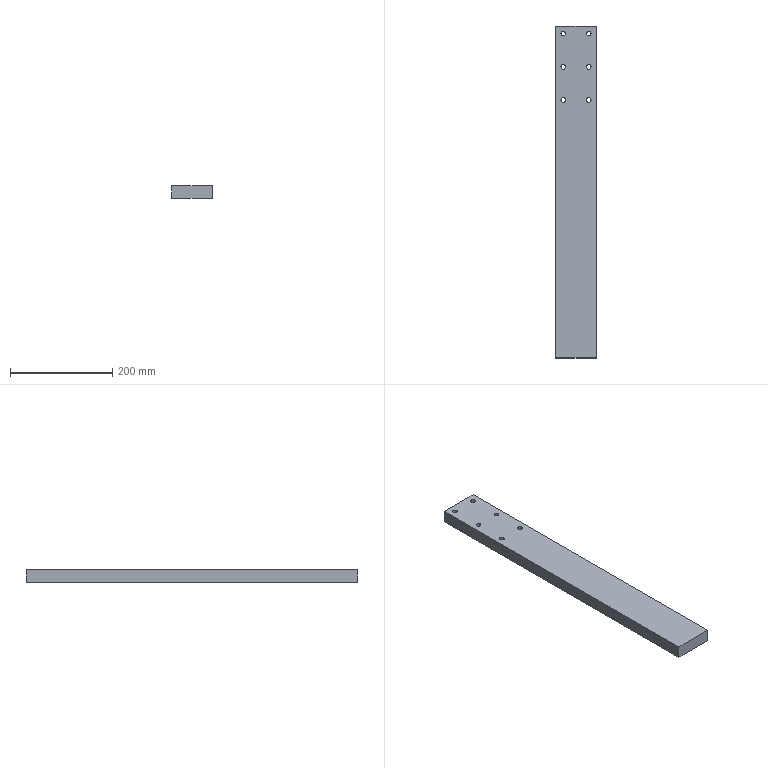Part | SolidWorks | features HoleWzd 2, 3DProfileFeature 1, Extrusion 1, LPattern 1 | 1 solid | 34 faces | box 80 x 650 x 25 mm | volume 1287489 mm3 | cylinder 20 | cone 8 | plane 6 | commonest cylinder face diameters 9 x12 6.8 x8
STEP:
#1=CARTESIAN_POINT('',(60.25,285.,15.9));
#2=VERTEX_POINT('',#1);
#3=CARTESIAN_POINT('',(60.25,285.,9.1));
#4=VERTEX_POINT('',#3);
#5=CARTESIAN_POINT('',(60.25,285.,12.5));
#6=DIRECTION('',(1.,0.,0.));
#7=DIRECTION('',(0.,0.,-1.));
#8=AXIS2_PLACEMENT_3D('',#5,#6,#7);
#9=CIRCLE('',#8,3.4);
#10=EDGE_CURVE('',#2,#4,#9,.T.);
#11=ORIENTED_EDGE('',*,*,#10,.F.);
#12=CARTESIAN_POINT('',(80.,285.,15.9));
#13=VERTEX_POINT('',#12);
#14=CARTESIAN_POINT('',(80.,285.,15.9));
#15=DIRECTION('',(1.,0.,0.));
#16=VECTOR('',#15,1000.);
#17=LINE('',#14,#16);
#18=EDGE_CURVE('',#2,#13,#17,.T.);
#19=ORIENTED_EDGE('',*,*,#18,.T.);
#20=CARTESIAN_POINT('',(80.,285.,9.1));
#21=VERTEX_POINT('',#20);
#22=CARTESIAN_POINT('',(80.,285.,12.5));
#23=DIRECTION('',(1.,0.,0.));
#24=DIRECTION('',(0.,0.,-1.));
#25=AXIS2_PLACEMENT_3D('',#22,#23,#24);
#26=CIRCLE('',#25,3.4);
#27=EDGE_CURVE('',#13,#21,#26,.T.);
#28=ORIENTED_EDGE('',*,*,#27,.T.);
#29=CARTESIAN_POINT('',(80.,285.,9.1));
#30=DIRECTION('',(1.,0.,0.));
#31=VECTOR('',#30,1000.);
#32=LINE('',#29,#31);
#33=EDGE_CURVE('',#4,#21,#32,.T.);
#34=ORIENTED_EDGE('',*,*,#33,.F.);
#35=EDGE_LOOP('',(#11,#19,#28,#34));
#36=FACE_OUTER_BOUND('',#35,.T.);
#37=CARTESIAN_POINT('',(80.,285.,12.5));
#38=DIRECTION('',(1.,0.,0.));
#39=DIRECTION('',(0.,0.,-1.));
#40=AXIS2_PLACEMENT_3D('',#37,#38,#39);
#41=CYLINDRICAL_SURFACE('',#40,3.4);
#42=ADVANCED_FACE('',(#36),#41,.F.);
#43=CARTESIAN_POINT('',(58.207,285.,12.5));
#44=VERTEX_POINT('',#43);
#45=CARTESIAN_POINT('',(60.25,285.,9.1));
#46=DIRECTION('',(0.515,0.,-0.8572));
#47=VECTOR('',#46,1000.);
#48=LINE('',#45,#47);
#49=EDGE_CURVE('',#44,#4,#48,.T.);
#50=ORIENTED_EDGE('',*,*,#49,.F.);
#51=CARTESIAN_POINT('',(60.25,285.,15.9));
#52=DIRECTION('',(0.515,0.,0.8572));
#53=VECTOR('',#52,1000.);
#54=LINE('',#51,#53);
#55=EDGE_CURVE('',#44,#2,#54,.T.);
#56=ORIENTED_EDGE('',*,*,#55,.T.);
#57=ORIENTED_EDGE('',*,*,#10,.T.);
#58=EDGE_LOOP('',(#50,#56,#57));
#59=FACE_OUTER_BOUND('',#58,.T.);
#60=CARTESIAN_POINT('',(60.25,285.,12.5));
#61=DIRECTION('',(1.,0.,0.));
#62=DIRECTION('',(0.,0.,-1.));
#63=AXIS2_PLACEMENT_3D('',#60,#61,#62);
#64=CONICAL_SURFACE('',#63,3.4,1.03);
#65=ADVANCED_FACE('',(#59),#64,.F.);
#66=CARTESIAN_POINT('',(60.25,320.,15.9));
#67=VERTEX_POINT('',#66);
#68=CARTESIAN_POINT('',(60.25,320.,9.1));
#69=VERTEX_POINT('',#68);
#70=CARTESIAN_POINT('',(60.25,320.,12.5));
#71=DIRECTION('',(1.,0.,0.));
#72=DIRECTION('',(0.,0.,-1.));
#73=AXIS2_PLACEMENT_3D('',#70,#71,#72);
#74=CIRCLE('',#73,3.4);
#75=EDGE_CURVE('',#67,#69,#74,.T.);
#76=ORIENTED_EDGE('',*,*,#75,.F.);
#77=CARTESIAN_POINT('',(80.,320.,15.9));
#78=VERTEX_POINT('',#77);
#79=CARTESIAN_POINT('',(80.,320.,15.9));
#80=DIRECTION('',(1.,0.,0.));
#81=VECTOR('',#80,1000.);
#82=LINE('',#79,#81);
#83=EDGE_CURVE('',#67,#78,#82,.T.);
#84=ORIENTED_EDGE('',*,*,#83,.T.);
#85=CARTESIAN_POINT('',(80.,320.,9.1));
#86=VERTEX_POINT('',#85);
#87=CARTESIAN_POINT('',(80.,320.,12.5));
#88=DIRECTION('',(1.,0.,0.));
#89=DIRECTION('',(0.,0.,-1.));
#90=AXIS2_PLACEMENT_3D('',#87,#88,#89);
#91=CIRCLE('',#90,3.4);
#92=EDGE_CURVE('',#78,#86,#91,.T.);
#93=ORIENTED_EDGE('',*,*,#92,.T.);
#94=CARTESIAN_POINT('',(80.,320.,9.1));
#95=DIRECTION('',(1.,0.,0.));
#96=VECTOR('',#95,1000.);
#97=LINE('',#94,#96);
#98=EDGE_CURVE('',#69,#86,#97,.T.);
#99=ORIENTED_EDGE('',*,*,#98,.F.);
#100=EDGE_LOOP('',(#76,#84,#93,#99));
#101=FACE_OUTER_BOUND('',#100,.T.);
#102=CARTESIAN_POINT('',(80.,320.,12.5));
#103=DIRECTION('',(1.,0.,0.));
#104=DIRECTION('',(0.,0.,-1.));
#105=AXIS2_PLACEMENT_3D('',#102,#103,#104);
#106=CYLINDRICAL_SURFACE('',#105,3.4);
#107=ADVANCED_FACE('',(#101),#106,.F.);
#108=CARTESIAN_POINT('',(58.207,320.,12.5));
#109=VERTEX_POINT('',#108);
#110=CARTESIAN_POINT('',(60.25,320.,9.1));
#111=DIRECTION('',(0.515,0.,-0.8572));
#112=VECTOR('',#111,1000.);
#113=LINE('',#110,#112);
#114=EDGE_CURVE('',#109,#69,#113,.T.);
#115=ORIENTED_EDGE('',*,*,#114,.F.);
#116=CARTESIAN_POINT('',(60.25,320.,15.9));
#117=DIRECTION('',(0.515,0.,0.8572));
#118=VECTOR('',#117,1000.);
#119=LINE('',#116,#118);
#120=EDGE_CURVE('',#109,#67,#119,.T.);
#121=ORIENTED_EDGE('',*,*,#120,.T.);
#122=ORIENTED_EDGE('',*,*,#75,.T.);
#123=EDGE_LOOP('',(#115,#121,#122));
#124=FACE_OUTER_BOUND('',#123,.T.);
#125=CARTESIAN_POINT('',(60.25,320.,12.5));
#126=DIRECTION('',(1.,0.,0.));
#127=DIRECTION('',(0.,0.,-1.));
#128=AXIS2_PLACEMENT_3D('',#125,#126,#127);
#129=CONICAL_SURFACE('',#128,3.4,1.03);
#130=ADVANCED_FACE('',(#124),#129,.F.);
#131=CARTESIAN_POINT('',(60.25,620.,15.9));
#132=VERTEX_POINT('',#131);
#133=CARTESIAN_POINT('',(60.25,620.,9.1));
#134=VERTEX_POINT('',#133);
#135=CARTESIAN_POINT('',(60.25,620.,12.5));
#136=DIRECTION('',(1.,0.,0.));
#137=DIRECTION('',(0.,0.,-1.));
#138=AXIS2_PLACEMENT_3D('',#135,#136,#137);
#139=CIRCLE('',#138,3.4);
#140=EDGE_CURVE('',#132,#134,#139,.T.);
#141=ORIENTED_EDGE('',*,*,#140,.F.);
#142=CARTESIAN_POINT('',(80.,620.,15.9));
#143=VERTEX_POINT('',#142);
#144=CARTESIAN_POINT('',(80.,620.,15.9));
#145=DIRECTION('',(1.,0.,0.));
#146=VECTOR('',#145,1000.);
#147=LINE('',#144,#146);
#148=EDGE_CURVE('',#132,#143,#147,.T.);
#149=ORIENTED_EDGE('',*,*,#148,.T.);
#150=CARTESIAN_POINT('',(80.,620.,9.1));
#151=VERTEX_POINT('',#150);
#152=CARTESIAN_POINT('',(80.,620.,12.5));
#153=DIRECTION('',(1.,0.,0.));
#154=DIRECTION('',(0.,0.,-1.));
#155=AXIS2_PLACEMENT_3D('',#152,#153,#154);
#156=CIRCLE('',#155,3.4);
#157=EDGE_CURVE('',#143,#151,#156,.T.);
#158=ORIENTED_EDGE('',*,*,#157,.T.);
#159=CARTESIAN_POINT('',(80.,620.,9.1));
#160=DIRECTION('',(1.,0.,0.));
#161=VECTOR('',#160,1000.);
#162=LINE('',#159,#161);
#163=EDGE_CURVE('',#134,#151,#162,.T.);
#164=ORIENTED_EDGE('',*,*,#163,.F.);
#165=EDGE_LOOP('',(#141,#149,#158,#164));
#166=FACE_OUTER_BOUND('',#165,.T.);
#167=CARTESIAN_POINT('',(80.,620.,12.5));
#168=DIRECTION('',(1.,0.,0.));
#169=DIRECTION('',(0.,0.,-1.));
#170=AXIS2_PLACEMENT_3D('',#167,#168,#169);
#171=CYLINDRICAL_SURFACE('',#170,3.4);
#172=ADVANCED_FACE('',(#166),#171,.F.);
#173=CARTESIAN_POINT('',(58.207,620.,12.5));
#174=VERTEX_POINT('',#173);
#175=CARTESIAN_POINT('',(60.25,620.,9.1));
#176=DIRECTION('',(0.515,0.,-0.8572));
#177=VECTOR('',#176,1000.);
#178=LINE('',#175,#177);
#179=EDGE_CURVE('',#174,#134,#178,.T.);
#180=ORIENTED_EDGE('',*,*,#179,.F.);
#181=CARTESIAN_POINT('',(60.25,620.,15.9));
#182=DIRECTION('',(0.515,0.,0.8572));
#183=VECTOR('',#182,1000.);
#184=LINE('',#181,#183);
#185=EDGE_CURVE('',#174,#132,#184,.T.);
#186=ORIENTED_EDGE('',*,*,#185,.T.);
#187=ORIENTED_EDGE('',*,*,#140,.T.);
#188=EDGE_LOOP('',(#180,#186,#187));
#189=FACE_OUTER_BOUND('',#188,.T.);
#190=CARTESIAN_POINT('',(60.25,620.,12.5));
#191=DIRECTION('',(1.,0.,0.));
#192=DIRECTION('',(0.,0.,-1.));
#193=AXIS2_PLACEMENT_3D('',#190,#191,#192);
#194=CONICAL_SURFACE('',#193,3.4,1.03);
#195=ADVANCED_FACE('',(#189),#194,.F.);
#196=CARTESIAN_POINT('',(60.25,585.,15.9));
#197=VERTEX_POINT('',#196);
#198=CARTESIAN_POINT('',(60.25,585.,9.1));
#199=VERTEX_POINT('',#198);
#200=CARTESIAN_POINT('',(60.25,585.,12.5));
#201=DIRECTION('',(1.,0.,0.));
#202=DIRECTION('',(0.,0.,-1.));
#203=AXIS2_PLACEMENT_3D('',#200,#201,#202);
#204=CIRCLE('',#203,3.4);
#205=EDGE_CURVE('',#197,#199,#204,.T.);
#206=ORIENTED_EDGE('',*,*,#205,.F.);
#207=CARTESIAN_POINT('',(80.,585.,15.9));
#208=VERTEX_POINT('',#207);
#209=CARTESIAN_POINT('',(80.,585.,15.9));
#210=DIRECTION('',(1.,0.,0.));
#211=VECTOR('',#210,1000.);
#212=LINE('',#209,#211);
#213=EDGE_CURVE('',#197,#208,#212,.T.);
#214=ORIENTED_EDGE('',*,*,#213,.T.);
#215=CARTESIAN_POINT('',(80.,585.,9.1));
#216=VERTEX_POINT('',#215);
#217=CARTESIAN_POINT('',(80.,585.,12.5));
#218=DIRECTION('',(1.,0.,0.));
#219=DIRECTION('',(0.,0.,-1.));
#220=AXIS2_PLACEMENT_3D('',#217,#218,#219);
#221=CIRCLE('',#220,3.4);
#222=EDGE_CURVE('',#208,#216,#221,.T.);
#223=ORIENTED_EDGE('',*,*,#222,.T.);
#224=CARTESIAN_POINT('',(80.,585.,9.1));
#225=DIRECTION('',(1.,0.,0.));
#226=VECTOR('',#225,1000.);
#227=LINE('',#224,#226);
#228=EDGE_CURVE('',#199,#216,#227,.T.);
#229=ORIENTED_EDGE('',*,*,#228,.F.);
#230=EDGE_LOOP('',(#206,#214,#223,#229));
#231=FACE_OUTER_BOUND('',#230,.T.);
#232=CARTESIAN_POINT('',(80.,585.,12.5));
#233=DIRECTION('',(1.,0.,0.));
#234=DIRECTION('',(0.,0.,-1.));
#235=AXIS2_PLACEMENT_3D('',#232,#233,#234);
#236=CYLINDRICAL_SURFACE('',#235,3.4);
#237=ADVANCED_FACE('',(#231),#236,.F.);
#238=CARTESIAN_POINT('',(58.207,585.,12.5));
#239=VERTEX_POINT('',#238);
#240=CARTESIAN_POINT('',(60.25,585.,9.1));
#241=DIRECTION('',(0.515,0.,-0.8572));
#242=VECTOR('',#241,1000.);
#243=LINE('',#240,#242);
#244=EDGE_CURVE('',#239,#199,#243,.T.);
#245=ORIENTED_EDGE('',*,*,#244,.F.);
#246=CARTESIAN_POINT('',(60.25,585.,15.9));
#247=DIRECTION('',(0.515,0.,0.8572));
#248=VECTOR('',#247,1000.);
#249=LINE('',#246,#248);
#250=EDGE_CURVE('',#239,#197,#249,.T.);
#251=ORIENTED_EDGE('',*,*,#250,.T.);
#252=ORIENTED_EDGE('',*,*,#205,.T.);
#253=EDGE_LOOP('',(#245,#251,#252));
#254=FACE_OUTER_BOUND('',#253,.T.);
#255=CARTESIAN_POINT('',(60.25,585.,12.5));
#256=DIRECTION('',(1.,0.,0.));
#257=DIRECTION('',(0.,0.,-1.));
#258=AXIS2_PLACEMENT_3D('',#255,#256,#257);
#259=CONICAL_SURFACE('',#258,3.4,1.03);
#260=ADVANCED_FACE('',(#254),#259,.F.);
#261=CARTESIAN_POINT('',(10.5,635.,0.));
#262=VERTEX_POINT('',#261);
#263=CARTESIAN_POINT('',(19.5,635.,0.));
#264=VERTEX_POINT('',#263);
#265=CARTESIAN_POINT('',(15.,635.,0.));
#266=DIRECTION('',(0.,0.,1.));
#267=DIRECTION('',(1.,0.,0.));
#268=AXIS2_PLACEMENT_3D('',#265,#266,#267);
#269=CIRCLE('',#268,4.5);
#270=EDGE_CURVE('',#262,#264,#269,.T.);
#271=ORIENTED_EDGE('',*,*,#270,.F.);
#272=CARTESIAN_POINT('',(10.5,635.,25.));
#273=VERTEX_POINT('',#272);
#274=CARTESIAN_POINT('',(10.5,635.,25.));
#275=DIRECTION('',(0.,0.,1.));
#276=VECTOR('',#275,1000.);
#277=LINE('',#274,#276);
#278=EDGE_CURVE('',#262,#273,#277,.T.);
#279=ORIENTED_EDGE('',*,*,#278,.T.);
#280=CARTESIAN_POINT('',(19.5,635.,25.));
#281=VERTEX_POINT('',#280);
#282=CARTESIAN_POINT('',(15.,635.,25.));
#283=DIRECTION('',(0.,0.,1.));
#284=DIRECTION('',(1.,0.,0.));
#285=AXIS2_PLACEMENT_3D('',#282,#283,#284);
#286=CIRCLE('',#285,4.5);
#287=EDGE_CURVE('',#273,#281,#286,.T.);
#288=ORIENTED_EDGE('',*,*,#287,.T.);
#289=CARTESIAN_POINT('',(19.5,635.,25.));
#290=DIRECTION('',(0.,0.,1.));
#291=VECTOR('',#290,1000.);
#292=LINE('',#289,#291);
#293=EDGE_CURVE('',#264,#281,#292,.T.);
#294=ORIENTED_EDGE('',*,*,#293,.F.);
#295=EDGE_LOOP('',(#271,#279,#288,#294));
#296=FACE_OUTER_BOUND('',#295,.T.);
#297=CARTESIAN_POINT('',(15.,635.,25.));
#298=DIRECTION('',(0.,0.,1.));
#299=DIRECTION('',(1.,0.,0.));
#300=AXIS2_PLACEMENT_3D('',#297,#298,#299);
#301=CYLINDRICAL_SURFACE('',#300,4.5);
#302=ADVANCED_FACE('',(#296),#301,.F.);
#303=CARTESIAN_POINT('',(60.5,635.,0.));
#304=VERTEX_POINT('',#303);
#305=CARTESIAN_POINT('',(69.5,635.,0.));
#306=VERTEX_POINT('',#305);
#307=CARTESIAN_POINT('',(65.,635.,0.));
#308=DIRECTION('',(0.,0.,1.));
#309=DIRECTION('',(1.,0.,0.));
#310=AXIS2_PLACEMENT_3D('',#307,#308,#309);
#311=CIRCLE('',#310,4.5);
#312=EDGE_CURVE('',#304,#306,#311,.T.);
#313=ORIENTED_EDGE('',*,*,#312,.F.);
#314=CARTESIAN_POINT('',(60.5,635.,25.));
#315=VERTEX_POINT('',#314);
#316=CARTESIAN_POINT('',(60.5,635.,25.));
#317=DIRECTION('',(0.,0.,1.));
#318=VECTOR('',#317,1000.);
#319=LINE('',#316,#318);
#320=EDGE_CURVE('',#304,#315,#319,.T.);
#321=ORIENTED_EDGE('',*,*,#320,.T.);
#322=CARTESIAN_POINT('',(69.5,635.,25.));
#323=VERTEX_POINT('',#322);
#324=CARTESIAN_POINT('',(65.,635.,25.));
#325=DIRECTION('',(0.,0.,1.));
#326=DIRECTION('',(1.,0.,0.));
#327=AXIS2_PLACEMENT_3D('',#324,#325,#326);
#328=CIRCLE('',#327,4.5);
#329=EDGE_CURVE('',#315,#323,#328,.T.);
#330=ORIENTED_EDGE('',*,*,#329,.T.);
#331=CARTESIAN_POINT('',(69.5,635.,25.));
#332=DIRECTION('',(0.,0.,1.));
#333=VECTOR('',#332,1000.);
#334=LINE('',#331,#333);
#335=EDGE_CURVE('',#306,#323,#334,.T.);
#336=ORIENTED_EDGE('',*,*,#335,.F.);
#337=EDGE_LOOP('',(#313,#321,#330,#336));
#338=FACE_OUTER_BOUND('',#337,.T.);
#339=CARTESIAN_POINT('',(65.,635.,25.));
#340=DIRECTION('',(0.,0.,1.));
#341=DIRECTION('',(1.,0.,0.));
#342=AXIS2_PLACEMENT_3D('',#339,#340,#341);
#343=CYLINDRICAL_SURFACE('',#342,4.5);
#344=ADVANCED_FACE('',(#338),#343,.F.);
#345=CARTESIAN_POINT('',(10.5,505.,0.));
#346=VERTEX_POINT('',#345);
#347=CARTESIAN_POINT('',(19.5,505.,0.));
#348=VERTEX_POINT('',#347);
#349=CARTESIAN_POINT('',(15.,505.,0.));
#350=DIRECTION('',(0.,0.,1.));
#351=DIRECTION('',(1.,0.,0.));
#352=AXIS2_PLACEMENT_3D('',#349,#350,#351);
#353=CIRCLE('',#352,4.5);
#354=EDGE_CURVE('',#346,#348,#353,.T.);
#355=ORIENTED_EDGE('',*,*,#354,.F.);
#356=CARTESIAN_POINT('',(10.5,505.,25.));
#357=VERTEX_POINT('',#356);
#358=CARTESIAN_POINT('',(10.5,505.,25.));
#359=DIRECTION('',(0.,0.,1.));
#360=VECTOR('',#359,1000.);
#361=LINE('',#358,#360);
#362=EDGE_CURVE('',#346,#357,#361,.T.);
#363=ORIENTED_EDGE('',*,*,#362,.T.);
#364=CARTESIAN_POINT('',(19.5,505.,25.));
#365=VERTEX_POINT('',#364);
#366=CARTESIAN_POINT('',(15.,505.,25.));
#367=DIRECTION('',(0.,0.,1.));
#368=DIRECTION('',(1.,0.,0.));
#369=AXIS2_PLACEMENT_3D('',#366,#367,#368);
#370=CIRCLE('',#369,4.5);
#371=EDGE_CURVE('',#357,#365,#370,.T.);
#372=ORIENTED_EDGE('',*,*,#371,.T.);
#373=CARTESIAN_POINT('',(19.5,505.,25.));
#374=DIRECTION('',(0.,0.,1.));
#375=VECTOR('',#374,1000.);
#376=LINE('',#373,#375);
#377=EDGE_CURVE('',#348,#365,#376,.T.);
#378=ORIENTED_EDGE('',*,*,#377,.F.);
#379=EDGE_LOOP('',(#355,#363,#372,#378));
#380=FACE_OUTER_BOUND('',#379,.T.);
#381=CARTESIAN_POINT('',(15.,505.,25.));
#382=DIRECTION('',(0.,0.,1.));
#383=DIRECTION('',(1.,0.,0.));
#384=AXIS2_PLACEMENT_3D('',#381,#382,#383);
#385=CYLINDRICAL_SURFACE('',#384,4.5);
#386=ADVANCED_FACE('',(#380),#385,.F.);
#387=CARTESIAN_POINT('',(60.5,505.,0.));
#388=VERTEX_POINT('',#387);
#389=CARTESIAN_POINT('',(69.5,505.,0.));
#390=VERTEX_POINT('',#389);
#391=CARTESIAN_POINT('',(65.,505.,0.));
#392=DIRECTION('',(0.,0.,1.));
#393=DIRECTION('',(1.,0.,0.));
#394=AXIS2_PLACEMENT_3D('',#391,#392,#393);
#395=CIRCLE('',#394,4.5);
#396=EDGE_CURVE('',#388,#390,#395,.T.);
#397=ORIENTED_EDGE('',*,*,#396,.F.);
#398=CARTESIAN_POINT('',(60.5,505.,25.));
#399=VERTEX_POINT('',#398);
#400=CARTESIAN_POINT('',(60.5,505.,25.));
#401=DIRECTION('',(0.,0.,1.));
#402=VECTOR('',#401,1000.);
#403=LINE('',#400,#402);
#404=EDGE_CURVE('',#388,#399,#403,.T.);
#405=ORIENTED_EDGE('',*,*,#404,.T.);
#406=CARTESIAN_POINT('',(69.5,505.,25.));
#407=VERTEX_POINT('',#406);
#408=CARTESIAN_POINT('',(65.,505.,25.));
#409=DIRECTION('',(0.,0.,1.));
#410=DIRECTION('',(1.,0.,0.));
#411=AXIS2_PLACEMENT_3D('',#408,#409,#410);
#412=CIRCLE('',#411,4.5);
#413=EDGE_CURVE('',#399,#407,#412,.T.);
#414=ORIENTED_EDGE('',*,*,#413,.T.);
#415=CARTESIAN_POINT('',(69.5,505.,25.));
#416=DIRECTION('',(0.,0.,1.));
#417=VECTOR('',#416,1000.);
#418=LINE('',#415,#417);
#419=EDGE_CURVE('',#390,#407,#418,.T.);
#420=ORIENTED_EDGE('',*,*,#419,.F.);
#421=EDGE_LOOP('',(#397,#405,#414,#420));
#422=FACE_OUTER_BOUND('',#421,.T.);
#423=CARTESIAN_POINT('',(65.,505.,25.));
#424=DIRECTION('',(0.,0.,1.));
#425=DIRECTION('',(1.,0.,0.));
#426=AXIS2_PLACEMENT_3D('',#423,#424,#425);
#427=CYLINDRICAL_SURFACE('',#426,4.5);
#428=ADVANCED_FACE('',(#422),#427,.F.);
#429=CARTESIAN_POINT('',(10.5,570.,0.));
#430=VERTEX_POINT('',#429);
#431=CARTESIAN_POINT('',(19.5,570.,0.));
#432=VERTEX_POINT('',#431);
#433=CARTESIAN_POINT('',(15.,570.,0.));
#434=DIRECTION('',(0.,0.,1.));
#435=DIRECTION('',(1.,0.,0.));
#436=AXIS2_PLACEMENT_3D('',#433,#434,#435);
#437=CIRCLE('',#436,4.5);
#438=EDGE_CURVE('',#430,#432,#437,.T.);
#439=ORIENTED_EDGE('',*,*,#438,.F.);
#440=CARTESIAN_POINT('',(10.5,570.,25.));
#441=VERTEX_POINT('',#440);
#442=CARTESIAN_POINT('',(10.5,570.,25.));
#443=DIRECTION('',(0.,0.,1.));
#444=VECTOR('',#443,1000.);
#445=LINE('',#442,#444);
#446=EDGE_CURVE('',#430,#441,#445,.T.);
#447=ORIENTED_EDGE('',*,*,#446,.T.);
#448=CARTESIAN_POINT('',(19.5,570.,25.));
#449=VERTEX_POINT('',#448);
#450=CARTESIAN_POINT('',(15.,570.,25.));
#451=DIRECTION('',(0.,0.,1.));
#452=DIRECTION('',(1.,0.,0.));
#453=AXIS2_PLACEMENT_3D('',#450,#451,#452);
#454=CIRCLE('',#453,4.5);
#455=EDGE_CURVE('',#441,#449,#454,.T.);
#456=ORIENTED_EDGE('',*,*,#455,.T.);
#457=CARTESIAN_POINT('',(19.5,570.,25.));
#458=DIRECTION('',(0.,0.,1.));
#459=VECTOR('',#458,1000.);
#460=LINE('',#457,#459);
#461=EDGE_CURVE('',#432,#449,#460,.T.);
#462=ORIENTED_EDGE('',*,*,#461,.F.);
#463=EDGE_LOOP('',(#439,#447,#456,#462));
#464=FACE_OUTER_BOUND('',#463,.T.);
#465=CARTESIAN_POINT('',(15.,570.,25.));
#466=DIRECTION('',(0.,0.,1.));
#467=DIRECTION('',(1.,0.,0.));
#468=AXIS2_PLACEMENT_3D('',#465,#466,#467);
#469=CYLINDRICAL_SURFACE('',#468,4.5);
#470=ADVANCED_FACE('',(#464),#469,.F.);
#471=CARTESIAN_POINT('',(60.5,570.,0.));
#472=VERTEX_POINT('',#471);
#473=CARTESIAN_POINT('',(69.5,570.,0.));
#474=VERTEX_POINT('',#473);
#475=CARTESIAN_POINT('',(65.,570.,0.));
#476=DIRECTION('',(0.,0.,1.));
#477=DIRECTION('',(1.,0.,0.));
#478=AXIS2_PLACEMENT_3D('',#475,#476,#477);
#479=CIRCLE('',#478,4.5);
#480=EDGE_CURVE('',#472,#474,#479,.T.);
#481=ORIENTED_EDGE('',*,*,#480,.F.);
#482=CARTESIAN_POINT('',(60.5,570.,25.));
#483=VERTEX_POINT('',#482);
#484=CARTESIAN_POINT('',(60.5,570.,25.));
#485=DIRECTION('',(0.,0.,1.));
#486=VECTOR('',#485,1000.);
#487=LINE('',#484,#486);
#488=EDGE_CURVE('',#472,#483,#487,.T.);
#489=ORIENTED_EDGE('',*,*,#488,.T.);
#490=CARTESIAN_POINT('',(69.5,570.,25.));
#491=VERTEX_POINT('',#490);
#492=CARTESIAN_POINT('',(65.,570.,25.));
#493=DIRECTION('',(0.,0.,1.));
#494=DIRECTION('',(1.,0.,0.));
#495=AXIS2_PLACEMENT_3D('',#492,#493,#494);
#496=CIRCLE('',#495,4.5);
#497=EDGE_CURVE('',#483,#491,#496,.T.);
#498=ORIENTED_EDGE('',*,*,#497,.T.);
#499=CARTESIAN_POINT('',(69.5,570.,25.));
#500=DIRECTION('',(0.,0.,1.));
#501=VECTOR('',#500,1000.);
#502=LINE('',#499,#501);
#503=EDGE_CURVE('',#474,#491,#502,.T.);
#504=ORIENTED_EDGE('',*,*,#503,.F.);
#505=EDGE_LOOP('',(#481,#489,#498,#504));
#506=FACE_OUTER_BOUND('',#505,.T.);
#507=CARTESIAN_POINT('',(65.,570.,25.));
#508=DIRECTION('',(0.,0.,1.));
#509=DIRECTION('',(1.,0.,0.));
#510=AXIS2_PLACEMENT_3D('',#507,#508,#509);
#511=CYLINDRICAL_SURFACE('',#510,4.5);
#512=ADVANCED_FACE('',(#506),#511,.F.);
#513=CARTESIAN_POINT('',(0.,650.,0.));
#514=VERTEX_POINT('',#513);
#515=CARTESIAN_POINT('',(0.,0.,0.));
#516=VERTEX_POINT('',#515);
#517=CARTESIAN_POINT('',(0.,0.,0.));
#518=DIRECTION('',(0.,-1.,0.));
#519=VECTOR('',#518,1000.);
#520=LINE('',#517,#519);
#521=EDGE_CURVE('',#514,#516,#520,.T.);
#522=ORIENTED_EDGE('',*,*,#521,.T.);
#523=CARTESIAN_POINT('',(0.,0.,25.));
#524=VERTEX_POINT('',#523);
#525=CARTESIAN_POINT('',(0.,0.,25.));
#526=DIRECTION('',(0.,0.,-1.));
#527=VECTOR('',#526,1000.);
#528=LINE('',#525,#527);
#529=EDGE_CURVE('',#524,#516,#528,.T.);
#530=ORIENTED_EDGE('',*,*,#529,.F.);
#531=CARTESIAN_POINT('',(0.,650.,25.));
#532=VERTEX_POINT('',#531);
#533=CARTESIAN_POINT('',(0.,0.,25.));
#534=DIRECTION('',(0.,-1.,0.));
#535=VECTOR('',#534,1000.);
#536=LINE('',#533,#535);
#537=EDGE_CURVE('',#532,#524,#536,.T.);
#538=ORIENTED_EDGE('',*,*,#537,.F.);
#539=CARTESIAN_POINT('',(0.,650.,25.));
#540=DIRECTION('',(0.,0.,-1.));
#541=VECTOR('',#540,1000.);
#542=LINE('',#539,#541);
#543=EDGE_CURVE('',#532,#514,#542,.T.);
#544=ORIENTED_EDGE('',*,*,#543,.T.);
#545=EDGE_LOOP('',(#522,#530,#538,#544));
#546=FACE_OUTER_BOUND('',#545,.T.);
#547=CARTESIAN_POINT('',(0.,0.,25.));
#548=DIRECTION('',(1.,0.,0.));
#549=DIRECTION('',(0.,0.,-1.));
#550=AXIS2_PLACEMENT_3D('',#547,#548,#549);
#551=PLANE('',#550);
#552=ADVANCED_FACE('',(#546),#551,.F.);
#553=CARTESIAN_POINT('',(80.,0.,0.));
#554=VERTEX_POINT('',#553);
#555=CARTESIAN_POINT('',(0.,0.,0.));
#556=DIRECTION('',(1.,0.,0.));
#557=VECTOR('',#556,1000.);
#558=LINE('',#555,#557);
#559=EDGE_CURVE('',#516,#554,#558,.T.);
#560=ORIENTED_EDGE('',*,*,#559,.T.);
#561=CARTESIAN_POINT('',(80.,0.,25.));
#562=VERTEX_POINT('',#561);
#563=CARTESIAN_POINT('',(80.,0.,25.));
#564=DIRECTION('',(0.,0.,-1.));
#565=VECTOR('',#564,1000.);
#566=LINE('',#563,#565);
#567=EDGE_CURVE('',#562,#554,#566,.T.);
#568=ORIENTED_EDGE('',*,*,#567,.F.);
#569=CARTESIAN_POINT('',(0.,0.,25.));
#570=DIRECTION('',(1.,0.,0.));
#571=VECTOR('',#570,1000.);
#572=LINE('',#569,#571);
#573=EDGE_CURVE('',#524,#562,#572,.T.);
#574=ORIENTED_EDGE('',*,*,#573,.F.);
#575=ORIENTED_EDGE('',*,*,#529,.T.);
#576=EDGE_LOOP('',(#560,#568,#574,#575));
#577=FACE_OUTER_BOUND('',#576,.T.);
#578=CARTESIAN_POINT('',(0.,0.,25.));
#579=DIRECTION('',(0.,1.,0.));
#580=DIRECTION('',(0.,0.,1.));
#581=AXIS2_PLACEMENT_3D('',#578,#579,#580);
#582=PLANE('',#581);
#583=ADVANCED_FACE('',(#577),#582,.F.);
#584=CARTESIAN_POINT('',(80.,285.,12.5));
#585=DIRECTION('',(1.,0.,0.));
#586=DIRECTION('',(0.,0.,-1.));
#587=AXIS2_PLACEMENT_3D('',#584,#585,#586);
#588=CIRCLE('',#587,3.4);
#589=EDGE_CURVE('',#21,#13,#588,.T.);
#590=ORIENTED_EDGE('',*,*,#589,.F.);
#591=ORIENTED_EDGE('',*,*,#27,.F.);
#592=EDGE_LOOP('',(#590,#591));
#593=FACE_BOUND('',#592,.T.);
#594=CARTESIAN_POINT('',(80.,320.,12.5));
#595=DIRECTION('',(1.,0.,0.));
#596=DIRECTION('',(0.,0.,-1.));
#597=AXIS2_PLACEMENT_3D('',#594,#595,#596);
#598=CIRCLE('',#597,3.4);
#599=EDGE_CURVE('',#86,#78,#598,.T.);
#600=ORIENTED_EDGE('',*,*,#599,.F.);
#601=ORIENTED_EDGE('',*,*,#92,.F.);
#602=EDGE_LOOP('',(#600,#601));
#603=FACE_BOUND('',#602,.T.);
#604=CARTESIAN_POINT('',(80.,620.,12.5));
#605=DIRECTION('',(1.,0.,0.));
#606=DIRECTION('',(0.,0.,-1.));
#607=AXIS2_PLACEMENT_3D('',#604,#605,#606);
#608=CIRCLE('',#607,3.4);
#609=EDGE_CURVE('',#151,#143,#608,.T.);
#610=ORIENTED_EDGE('',*,*,#609,.F.);
#611=ORIENTED_EDGE('',*,*,#157,.F.);
#612=EDGE_LOOP('',(#610,#611));
#613=FACE_BOUND('',#612,.T.);
#614=CARTESIAN_POINT('',(80.,585.,12.5));
#615=DIRECTION('',(1.,0.,0.));
#616=DIRECTION('',(0.,0.,-1.));
#617=AXIS2_PLACEMENT_3D('',#614,#615,#616);
#618=CIRCLE('',#617,3.4);
#619=EDGE_CURVE('',#216,#208,#618,.T.);
#620=ORIENTED_EDGE('',*,*,#619,.F.);
#621=ORIENTED_EDGE('',*,*,#222,.F.);
#622=EDGE_LOOP('',(#620,#621));
#623=FACE_BOUND('',#622,.T.);
#624=CARTESIAN_POINT('',(80.,650.,0.));
#625=VERTEX_POINT('',#624);
#626=CARTESIAN_POINT('',(80.,80.,0.));
#627=DIRECTION('',(0.,1.,0.));
#628=VECTOR('',#627,1000.);
#629=LINE('',#626,#628);
#630=EDGE_CURVE('',#554,#625,#629,.T.);
#631=ORIENTED_EDGE('',*,*,#630,.T.);
#632=CARTESIAN_POINT('',(80.,650.,25.));
#633=VERTEX_POINT('',#632);
#634=CARTESIAN_POINT('',(80.,650.,25.));
#635=DIRECTION('',(0.,0.,-1.));
#636=VECTOR('',#635,1000.);
#637=LINE('',#634,#636);
#638=EDGE_CURVE('',#633,#625,#637,.T.);
#639=ORIENTED_EDGE('',*,*,#638,.F.);
#640=CARTESIAN_POINT('',(80.,0.,25.));
#641=DIRECTION('',(0.,1.,0.));
#642=VECTOR('',#641,1000.);
#643=LINE('',#640,#642);
#644=EDGE_CURVE('',#562,#633,#643,.T.);
#645=ORIENTED_EDGE('',*,*,#644,.F.);
#646=ORIENTED_EDGE('',*,*,#567,.T.);
#647=EDGE_LOOP('',(#631,#639,#645,#646));
#648=FACE_OUTER_BOUND('',#647,.T.);
#649=CARTESIAN_POINT('',(80.,80.,25.));
#650=DIRECTION('',(-1.,0.,0.));
#651=DIRECTION('',(0.,0.,1.));
#652=AXIS2_PLACEMENT_3D('',#649,#650,#651);
#653=PLANE('',#652);
#654=ADVANCED_FACE('',(#593,#603,#613,#623,#648),#653,.F.);
#655=CARTESIAN_POINT('',(0.,650.,0.));
#656=DIRECTION('',(-1.,0.,0.));
#657=VECTOR('',#656,1000.);
#658=LINE('',#655,#657);
#659=EDGE_CURVE('',#625,#514,#658,.T.);
#660=ORIENTED_EDGE('',*,*,#659,.T.);
#661=ORIENTED_EDGE('',*,*,#543,.F.);
#662=CARTESIAN_POINT('',(0.,650.,25.));
#663=DIRECTION('',(-1.,0.,0.));
#664=VECTOR('',#663,1000.);
#665=LINE('',#662,#664);
#666=EDGE_CURVE('',#633,#532,#665,.T.);
#667=ORIENTED_EDGE('',*,*,#666,.F.);
#668=ORIENTED_EDGE('',*,*,#638,.T.);
#669=EDGE_LOOP('',(#660,#661,#667,#668));
#670=FACE_OUTER_BOUND('',#669,.T.);
#671=CARTESIAN_POINT('',(0.,650.,25.));
#672=DIRECTION('',(0.,-1.,0.));
#673=DIRECTION('',(0.,0.,-1.));
#674=AXIS2_PLACEMENT_3D('',#671,#672,#673);
#675=PLANE('',#674);
#676=ADVANCED_FACE('',(#670),#675,.F.);
#677=CARTESIAN_POINT('',(15.,635.,25.));
#678=DIRECTION('',(0.,0.,1.));
#679=DIRECTION('',(1.,0.,0.));
#680=AXIS2_PLACEMENT_3D('',#677,#678,#679);
#681=CIRCLE('',#680,4.5);
#682=EDGE_CURVE('',#281,#273,#681,.T.);
#683=ORIENTED_EDGE('',*,*,#682,.F.);
#684=ORIENTED_EDGE('',*,*,#287,.F.);
#685=EDGE_LOOP('',(#683,#684));
#686=FACE_BOUND('',#685,.T.);
#687=CARTESIAN_POINT('',(65.,635.,25.));
#688=DIRECTION('',(0.,0.,1.));
#689=DIRECTION('',(1.,0.,0.));
#690=AXIS2_PLACEMENT_3D('',#687,#688,#689);
#691=CIRCLE('',#690,4.5);
#692=EDGE_CURVE('',#323,#315,#691,.T.);
#693=ORIENTED_EDGE('',*,*,#692,.F.);
#694=ORIENTED_EDGE('',*,*,#329,.F.);
#695=EDGE_LOOP('',(#693,#694));
#696=FACE_BOUND('',#695,.T.);
#697=CARTESIAN_POINT('',(15.,505.,25.));
#698=DIRECTION('',(0.,0.,1.));
#699=DIRECTION('',(1.,0.,0.));
#700=AXIS2_PLACEMENT_3D('',#697,#698,#699);
#701=CIRCLE('',#700,4.5);
#702=EDGE_CURVE('',#365,#357,#701,.T.);
#703=ORIENTED_EDGE('',*,*,#702,.F.);
#704=ORIENTED_EDGE('',*,*,#371,.F.);
#705=EDGE_LOOP('',(#703,#704));
#706=FACE_BOUND('',#705,.T.);
#707=CARTESIAN_POINT('',(65.,505.,25.));
#708=DIRECTION('',(0.,0.,1.));
#709=DIRECTION('',(1.,0.,0.));
#710=AXIS2_PLACEMENT_3D('',#707,#708,#709);
#711=CIRCLE('',#710,4.5);
#712=EDGE_CURVE('',#407,#399,#711,.T.);
#713=ORIENTED_EDGE('',*,*,#712,.F.);
#714=ORIENTED_EDGE('',*,*,#413,.F.);
#715=EDGE_LOOP('',(#713,#714));
#716=FACE_BOUND('',#715,.T.);
#717=CARTESIAN_POINT('',(15.,570.,25.));
#718=DIRECTION('',(0.,0.,1.));
#719=DIRECTION('',(1.,0.,0.));
#720=AXIS2_PLACEMENT_3D('',#717,#718,#719);
#721=CIRCLE('',#720,4.5);
#722=EDGE_CURVE('',#449,#441,#721,.T.);
#723=ORIENTED_EDGE('',*,*,#722,.F.);
#724=ORIENTED_EDGE('',*,*,#455,.F.);
#725=EDGE_LOOP('',(#723,#724));
#726=FACE_BOUND('',#725,.T.);
#727=CARTESIAN_POINT('',(65.,570.,25.));
#728=DIRECTION('',(0.,0.,1.));
#729=DIRECTION('',(1.,0.,0.));
#730=AXIS2_PLACEMENT_3D('',#727,#728,#729);
#731=CIRCLE('',#730,4.5);
#732=EDGE_CURVE('',#491,#483,#731,.T.);
#733=ORIENTED_EDGE('',*,*,#732,.F.);
#734=ORIENTED_EDGE('',*,*,#497,.F.);
#735=EDGE_LOOP('',(#733,#734));
#736=FACE_BOUND('',#735,.T.);
#737=ORIENTED_EDGE('',*,*,#537,.T.);
#738=ORIENTED_EDGE('',*,*,#573,.T.);
#739=ORIENTED_EDGE('',*,*,#644,.T.);
#740=ORIENTED_EDGE('',*,*,#666,.T.);
#741=EDGE_LOOP('',(#737,#738,#739,#740));
#742=FACE_OUTER_BOUND('',#741,.T.);
#743=CARTESIAN_POINT('',(0.,0.,25.));
#744=DIRECTION('',(0.,0.,-1.));
#745=DIRECTION('',(-1.,0.,0.));
#746=AXIS2_PLACEMENT_3D('',#743,#744,#745);
#747=PLANE('',#746);
#748=ADVANCED_FACE('',(#686,#696,#706,#716,#726,#736,#742),#747,.F.);
#749=CARTESIAN_POINT('',(15.,635.,0.));
#750=DIRECTION('',(0.,0.,1.));
#751=DIRECTION('',(1.,0.,0.));
#752=AXIS2_PLACEMENT_3D('',#749,#750,#751);
#753=CIRCLE('',#752,4.5);
#754=EDGE_CURVE('',#264,#262,#753,.T.);
#755=ORIENTED_EDGE('',*,*,#754,.T.);
#756=ORIENTED_EDGE('',*,*,#270,.T.);
#757=EDGE_LOOP('',(#755,#756));
#758=FACE_BOUND('',#757,.T.);
#759=CARTESIAN_POINT('',(65.,635.,0.));
#760=DIRECTION('',(0.,0.,1.));
#761=DIRECTION('',(1.,0.,0.));
#762=AXIS2_PLACEMENT_3D('',#759,#760,#761);
#763=CIRCLE('',#762,4.5);
#764=EDGE_CURVE('',#306,#304,#763,.T.);
#765=ORIENTED_EDGE('',*,*,#764,.T.);
#766=ORIENTED_EDGE('',*,*,#312,.T.);
#767=EDGE_LOOP('',(#765,#766));
#768=FACE_BOUND('',#767,.T.);
#769=CARTESIAN_POINT('',(15.,505.,0.));
#770=DIRECTION('',(0.,0.,1.));
#771=DIRECTION('',(1.,0.,0.));
#772=AXIS2_PLACEMENT_3D('',#769,#770,#771);
#773=CIRCLE('',#772,4.5);
#774=EDGE_CURVE('',#348,#346,#773,.T.);
#775=ORIENTED_EDGE('',*,*,#774,.T.);
#776=ORIENTED_EDGE('',*,*,#354,.T.);
#777=EDGE_LOOP('',(#775,#776));
#778=FACE_BOUND('',#777,.T.);
#779=CARTESIAN_POINT('',(65.,505.,0.));
#780=DIRECTION('',(0.,0.,1.));
#781=DIRECTION('',(1.,0.,0.));
#782=AXIS2_PLACEMENT_3D('',#779,#780,#781);
#783=CIRCLE('',#782,4.5);
#784=EDGE_CURVE('',#390,#388,#783,.T.);
#785=ORIENTED_EDGE('',*,*,#784,.T.);
#786=ORIENTED_EDGE('',*,*,#396,.T.);
#787=EDGE_LOOP('',(#785,#786));
#788=FACE_BOUND('',#787,.T.);
#789=CARTESIAN_POINT('',(15.,570.,0.));
#790=DIRECTION('',(0.,0.,1.));
#791=DIRECTION('',(1.,0.,0.));
#792=AXIS2_PLACEMENT_3D('',#789,#790,#791);
#793=CIRCLE('',#792,4.5);
#794=EDGE_CURVE('',#432,#430,#793,.T.);
#795=ORIENTED_EDGE('',*,*,#794,.T.);
#796=ORIENTED_EDGE('',*,*,#438,.T.);
#797=EDGE_LOOP('',(#795,#796));
#798=FACE_BOUND('',#797,.T.);
#799=CARTESIAN_POINT('',(65.,570.,0.));
#800=DIRECTION('',(0.,0.,1.));
#801=DIRECTION('',(1.,0.,0.));
#802=AXIS2_PLACEMENT_3D('',#799,#800,#801);
#803=CIRCLE('',#802,4.5);
#804=EDGE_CURVE('',#474,#472,#803,.T.);
#805=ORIENTED_EDGE('',*,*,#804,.T.);
#806=ORIENTED_EDGE('',*,*,#480,.T.);
#807=EDGE_LOOP('',(#805,#806));
#808=FACE_BOUND('',#807,.T.);
#809=ORIENTED_EDGE('',*,*,#521,.F.);
#810=ORIENTED_EDGE('',*,*,#659,.F.);
#811=ORIENTED_EDGE('',*,*,#630,.F.);
#812=ORIENTED_EDGE('',*,*,#559,.F.);
#813=EDGE_LOOP('',(#809,#810,#811,#812));
#814=FACE_OUTER_BOUND('',#813,.T.);
#815=CARTESIAN_POINT('',(0.,0.,0.));
#816=DIRECTION('',(0.,0.,-1.));
#817=DIRECTION('',(-1.,0.,0.));
#818=AXIS2_PLACEMENT_3D('',#815,#816,#817);
#819=PLANE('',#818);
#820=ADVANCED_FACE('',(#758,#768,#778,#788,#798,#808,#814),#819,.T.);
#821=ORIENTED_EDGE('',*,*,#488,.F.);
#822=ORIENTED_EDGE('',*,*,#804,.F.);
#823=ORIENTED_EDGE('',*,*,#503,.T.);
#824=ORIENTED_EDGE('',*,*,#732,.T.);
#825=EDGE_LOOP('',(#821,#822,#823,#824));
#826=FACE_OUTER_BOUND('',#825,.T.);
#827=CARTESIAN_POINT('',(65.,570.,25.));
#828=DIRECTION('',(0.,0.,1.));
#829=DIRECTION('',(1.,0.,0.));
#830=AXIS2_PLACEMENT_3D('',#827,#828,#829);
#831=CYLINDRICAL_SURFACE('',#830,4.5);
#832=ADVANCED_FACE('',(#826),#831,.F.);
#833=ORIENTED_EDGE('',*,*,#446,.F.);
#834=ORIENTED_EDGE('',*,*,#794,.F.);
#835=ORIENTED_EDGE('',*,*,#461,.T.);
#836=ORIENTED_EDGE('',*,*,#722,.T.);
#837=EDGE_LOOP('',(#833,#834,#835,#836));
#838=FACE_OUTER_BOUND('',#837,.T.);
#839=CARTESIAN_POINT('',(15.,570.,25.));
#840=DIRECTION('',(0.,0.,1.));
#841=DIRECTION('',(1.,0.,0.));
#842=AXIS2_PLACEMENT_3D('',#839,#840,#841);
#843=CYLINDRICAL_SURFACE('',#842,4.5);
#844=ADVANCED_FACE('',(#838),#843,.F.);
#845=ORIENTED_EDGE('',*,*,#404,.F.);
#846=ORIENTED_EDGE('',*,*,#784,.F.);
#847=ORIENTED_EDGE('',*,*,#419,.T.);
#848=ORIENTED_EDGE('',*,*,#712,.T.);
#849=EDGE_LOOP('',(#845,#846,#847,#848));
#850=FACE_OUTER_BOUND('',#849,.T.);
#851=CARTESIAN_POINT('',(65.,505.,25.));
#852=DIRECTION('',(0.,0.,1.));
#853=DIRECTION('',(1.,0.,0.));
#854=AXIS2_PLACEMENT_3D('',#851,#852,#853);
#855=CYLINDRICAL_SURFACE('',#854,4.5);
#856=ADVANCED_FACE('',(#850),#855,.F.);
#857=ORIENTED_EDGE('',*,*,#362,.F.);
#858=ORIENTED_EDGE('',*,*,#774,.F.);
#859=ORIENTED_EDGE('',*,*,#377,.T.);
#860=ORIENTED_EDGE('',*,*,#702,.T.);
#861=EDGE_LOOP('',(#857,#858,#859,#860));
#862=FACE_OUTER_BOUND('',#861,.T.);
#863=CARTESIAN_POINT('',(15.,505.,25.));
#864=DIRECTION('',(0.,0.,1.));
#865=DIRECTION('',(1.,0.,0.));
#866=AXIS2_PLACEMENT_3D('',#863,#864,#865);
#867=CYLINDRICAL_SURFACE('',#866,4.5);
#868=ADVANCED_FACE('',(#862),#867,.F.);
#869=ORIENTED_EDGE('',*,*,#320,.F.);
#870=ORIENTED_EDGE('',*,*,#764,.F.);
#871=ORIENTED_EDGE('',*,*,#335,.T.);
#872=ORIENTED_EDGE('',*,*,#692,.T.);
#873=EDGE_LOOP('',(#869,#870,#871,#872));
#874=FACE_OUTER_BOUND('',#873,.T.);
#875=CARTESIAN_POINT('',(65.,635.,25.));
#876=DIRECTION('',(0.,0.,1.));
#877=DIRECTION('',(1.,0.,0.));
#878=AXIS2_PLACEMENT_3D('',#875,#876,#877);
#879=CYLINDRICAL_SURFACE('',#878,4.5);
#880=ADVANCED_FACE('',(#874),#879,.F.);
#881=ORIENTED_EDGE('',*,*,#278,.F.);
#882=ORIENTED_EDGE('',*,*,#754,.F.);
#883=ORIENTED_EDGE('',*,*,#293,.T.);
#884=ORIENTED_EDGE('',*,*,#682,.T.);
#885=EDGE_LOOP('',(#881,#882,#883,#884));
#886=FACE_OUTER_BOUND('',#885,.T.);
#887=CARTESIAN_POINT('',(15.,635.,25.));
#888=DIRECTION('',(0.,0.,1.));
#889=DIRECTION('',(1.,0.,0.));
#890=AXIS2_PLACEMENT_3D('',#887,#888,#889);
#891=CYLINDRICAL_SURFACE('',#890,4.5);
#892=ADVANCED_FACE('',(#886),#891,.F.);
#893=ORIENTED_EDGE('',*,*,#250,.F.);
#894=ORIENTED_EDGE('',*,*,#244,.T.);
#895=CARTESIAN_POINT('',(60.25,585.,12.5));
#896=DIRECTION('',(1.,0.,0.));
#897=DIRECTION('',(0.,0.,-1.));
#898=AXIS2_PLACEMENT_3D('',#895,#896,#897);
#899=CIRCLE('',#898,3.4);
#900=EDGE_CURVE('',#199,#197,#899,.T.);
#901=ORIENTED_EDGE('',*,*,#900,.T.);
#902=EDGE_LOOP('',(#893,#894,#901));
#903=FACE_OUTER_BOUND('',#902,.T.);
#904=CARTESIAN_POINT('',(60.25,585.,12.5));
#905=DIRECTION('',(1.,0.,0.));
#906=DIRECTION('',(0.,0.,-1.));
#907=AXIS2_PLACEMENT_3D('',#904,#905,#906);
#908=CONICAL_SURFACE('',#907,3.4,1.03);
#909=ADVANCED_FACE('',(#903),#908,.F.);
#910=ORIENTED_EDGE('',*,*,#213,.F.);
#911=ORIENTED_EDGE('',*,*,#900,.F.);
#912=ORIENTED_EDGE('',*,*,#228,.T.);
#913=ORIENTED_EDGE('',*,*,#619,.T.);
#914=EDGE_LOOP('',(#910,#911,#912,#913));
#915=FACE_OUTER_BOUND('',#914,.T.);
#916=CARTESIAN_POINT('',(80.,585.,12.5));
#917=DIRECTION('',(1.,0.,0.));
#918=DIRECTION('',(0.,0.,-1.));
#919=AXIS2_PLACEMENT_3D('',#916,#917,#918);
#920=CYLINDRICAL_SURFACE('',#919,3.4);
#921=ADVANCED_FACE('',(#915),#920,.F.);
#922=ORIENTED_EDGE('',*,*,#185,.F.);
#923=ORIENTED_EDGE('',*,*,#179,.T.);
#924=CARTESIAN_POINT('',(60.25,620.,12.5));
#925=DIRECTION('',(1.,0.,0.));
#926=DIRECTION('',(0.,0.,-1.));
#927=AXIS2_PLACEMENT_3D('',#924,#925,#926);
#928=CIRCLE('',#927,3.4);
#929=EDGE_CURVE('',#134,#132,#928,.T.);
#930=ORIENTED_EDGE('',*,*,#929,.T.);
#931=EDGE_LOOP('',(#922,#923,#930));
#932=FACE_OUTER_BOUND('',#931,.T.);
#933=CARTESIAN_POINT('',(60.25,620.,12.5));
#934=DIRECTION('',(1.,0.,0.));
#935=DIRECTION('',(0.,0.,-1.));
#936=AXIS2_PLACEMENT_3D('',#933,#934,#935);
#937=CONICAL_SURFACE('',#936,3.4,1.03);
#938=ADVANCED_FACE('',(#932),#937,.F.);
#939=ORIENTED_EDGE('',*,*,#148,.F.);
#940=ORIENTED_EDGE('',*,*,#929,.F.);
#941=ORIENTED_EDGE('',*,*,#163,.T.);
#942=ORIENTED_EDGE('',*,*,#609,.T.);
#943=EDGE_LOOP('',(#939,#940,#941,#942));
#944=FACE_OUTER_BOUND('',#943,.T.);
#945=CARTESIAN_POINT('',(80.,620.,12.5));
#946=DIRECTION('',(1.,0.,0.));
#947=DIRECTION('',(0.,0.,-1.));
#948=AXIS2_PLACEMENT_3D('',#945,#946,#947);
#949=CYLINDRICAL_SURFACE('',#948,3.4);
#950=ADVANCED_FACE('',(#944),#949,.F.);
#951=ORIENTED_EDGE('',*,*,#120,.F.);
#952=ORIENTED_EDGE('',*,*,#114,.T.);
#953=CARTESIAN_POINT('',(60.25,320.,12.5));
#954=DIRECTION('',(1.,0.,0.));
#955=DIRECTION('',(0.,0.,-1.));
#956=AXIS2_PLACEMENT_3D('',#953,#954,#955);
#957=CIRCLE('',#956,3.4);
#958=EDGE_CURVE('',#69,#67,#957,.T.);
#959=ORIENTED_EDGE('',*,*,#958,.T.);
#960=EDGE_LOOP('',(#951,#952,#959));
#961=FACE_OUTER_BOUND('',#960,.T.);
#962=CARTESIAN_POINT('',(60.25,320.,12.5));
#963=DIRECTION('',(1.,0.,0.));
#964=DIRECTION('',(0.,0.,-1.));
#965=AXIS2_PLACEMENT_3D('',#962,#963,#964);
#966=CONICAL_SURFACE('',#965,3.4,1.03);
#967=ADVANCED_FACE('',(#961),#966,.F.);
#968=ORIENTED_EDGE('',*,*,#83,.F.);
#969=ORIENTED_EDGE('',*,*,#958,.F.);
#970=ORIENTED_EDGE('',*,*,#98,.T.);
#971=ORIENTED_EDGE('',*,*,#599,.T.);
#972=EDGE_LOOP('',(#968,#969,#970,#971));
#973=FACE_OUTER_BOUND('',#972,.T.);
#974=CARTESIAN_POINT('',(80.,320.,12.5));
#975=DIRECTION('',(1.,0.,0.));
#976=DIRECTION('',(0.,0.,-1.));
#977=AXIS2_PLACEMENT_3D('',#974,#975,#976);
#978=CYLINDRICAL_SURFACE('',#977,3.4);
#979=ADVANCED_FACE('',(#973),#978,.F.);
#980=ORIENTED_EDGE('',*,*,#55,.F.);
#981=ORIENTED_EDGE('',*,*,#49,.T.);
#982=CARTESIAN_POINT('',(60.25,285.,12.5));
#983=DIRECTION('',(1.,0.,0.));
#984=DIRECTION('',(0.,0.,-1.));
#985=AXIS2_PLACEMENT_3D('',#982,#983,#984);
#986=CIRCLE('',#985,3.4);
#987=EDGE_CURVE('',#4,#2,#986,.T.);
#988=ORIENTED_EDGE('',*,*,#987,.T.);
#989=EDGE_LOOP('',(#980,#981,#988));
#990=FACE_OUTER_BOUND('',#989,.T.);
#991=CARTESIAN_POINT('',(60.25,285.,12.5));
#992=DIRECTION('',(1.,0.,0.));
#993=DIRECTION('',(0.,0.,-1.));
#994=AXIS2_PLACEMENT_3D('',#991,#992,#993);
#995=CONICAL_SURFACE('',#994,3.4,1.03);
#996=ADVANCED_FACE('',(#990),#995,.F.);
#997=ORIENTED_EDGE('',*,*,#18,.F.);
#998=ORIENTED_EDGE('',*,*,#987,.F.);
#999=ORIENTED_EDGE('',*,*,#33,.T.);
#1000=ORIENTED_EDGE('',*,*,#589,.T.);
#1001=EDGE_LOOP('',(#997,#998,#999,#1000));
#1002=FACE_OUTER_BOUND('',#1001,.T.);
#1003=CARTESIAN_POINT('',(80.,285.,12.5));
#1004=DIRECTION('',(1.,0.,0.));
#1005=DIRECTION('',(0.,0.,-1.));
#1006=AXIS2_PLACEMENT_3D('',#1003,#1004,#1005);
#1007=CYLINDRICAL_SURFACE('',#1006,3.4);
#1008=ADVANCED_FACE('',(#1002),#1007,.F.);
#1009=CLOSED_SHELL('',(#42,#65,#107,#130,#172,#195,#237,#260,#302,#344,#386,#428,#470,#512,#552,#583,#654,#676,#748,#820,#832,#844,#856,#868,#880,#892,#909,#921,#938,#950,#967,#979,#996,#1008));
#1010=MANIFOLD_SOLID_BREP('',#1009);
#1011=CARTESIAN_POINT('',(0.,0.,0.));
#1012=DIRECTION('',(0.,0.,1.));
#1013=DIRECTION('',(1.,0.,0.));
#1014=AXIS2_PLACEMENT_3D('',#1011,#1012,#1013);
#1015=(LENGTH_UNIT()NAMED_UNIT(*)SI_UNIT(.MILLI.,.METRE.));
#1016=UNCERTAINTY_MEASURE_WITH_UNIT(LENGTH_MEASURE(0.00001),#1015,'','');
#1017=(NAMED_UNIT(*)PLANE_ANGLE_UNIT()SI_UNIT($,.RADIAN.));
#1018=(NAMED_UNIT(*)SI_UNIT($,.STERADIAN.)SOLID_ANGLE_UNIT());
#1019=(GEOMETRIC_REPRESENTATION_CONTEXT(3)GLOBAL_UNCERTAINTY_ASSIGNED_CONTEXT((#1016))GLOBAL_UNIT_ASSIGNED_CONTEXT((#1015,#1017,#1018))REPRESENTATION_CONTEXT('',''));
#1020=ADVANCED_BREP_SHAPE_REPRESENTATION('',(#1010,#1014),#1019);